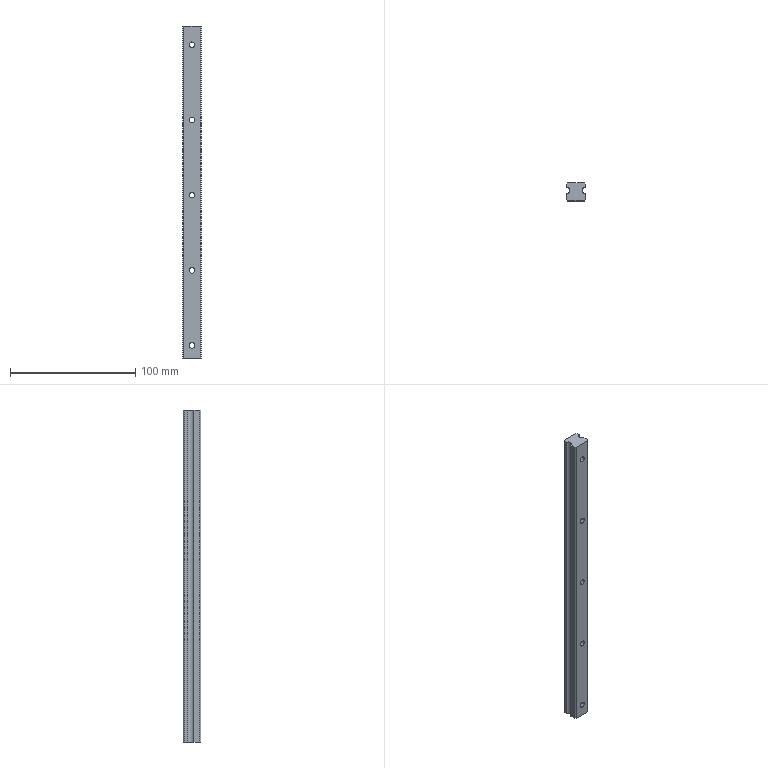Part | Creo | features CUT 6, CURVE 3, DATUM PLANE 3, COORDINATE SYSTEM 1, PATTERN 1, PROTRUSION 1 | 1 solid | 39 faces | box 15 x 14 x 265 mm | volume 47944 mm3 | cylinder 22 | plane 17 | commonest cylinder face diameters 4.5 x10 8 x10 5 x2
STEP:
#1=CARTESIAN_POINT('',(0.,0.,0.));
#2=DIRECTION('',(0.,0.,1.));
#3=DIRECTION('',(1.,0.,0.));
#4=AXIS2_PLACEMENT_3D('',#1,#2,#3);
#5=CARTESIAN_POINT('',(13.635,5.984,0.));
#6=VERTEX_POINT('',#5);
#7=CARTESIAN_POINT('',(13.635,10.984,0.));
#8=VERTEX_POINT('',#7);
#9=CARTESIAN_POINT('',(13.635,8.484,0.));
#10=DIRECTION('',(0.,0.,-1.));
#11=DIRECTION('',(0.00001575,-1.,0.));
#12=AXIS2_PLACEMENT_3D('',#9,#10,#11);
#13=CIRCLE('',#12,2.5);
#14=EDGE_CURVE('',#6,#8,#13,.T.);
#15=ORIENTED_EDGE('',*,*,#14,.T.);
#16=CARTESIAN_POINT('',(13.635,13.484,0.));
#17=VERTEX_POINT('',#16);
#18=CARTESIAN_POINT('',(13.635,10.984,0.));
#19=DIRECTION('',(-0.00001575,1.,0.));
#20=VECTOR('',#19,2.5);
#21=LINE('',#18,#20);
#22=EDGE_CURVE('',#8,#17,#21,.T.);
#23=ORIENTED_EDGE('',*,*,#22,.T.);
#24=CARTESIAN_POINT('',(12.635,14.484,0.));
#25=VERTEX_POINT('',#24);
#26=CARTESIAN_POINT('',(13.635,13.484,0.));
#27=DIRECTION('',(-0.7071,0.7071,0.));
#28=VECTOR('',#27,1.414);
#29=LINE('',#26,#28);
#30=EDGE_CURVE('',#17,#25,#29,.T.);
#31=ORIENTED_EDGE('',*,*,#30,.T.);
#32=CARTESIAN_POINT('',(-0.3654,14.484,0.));
#33=VERTEX_POINT('',#32);
#34=CARTESIAN_POINT('',(12.635,14.484,0.));
#35=DIRECTION('',(-1.,0.,0.));
#36=VECTOR('',#35,13.);
#37=LINE('',#34,#36);
#38=EDGE_CURVE('',#25,#33,#37,.T.);
#39=ORIENTED_EDGE('',*,*,#38,.T.);
#40=CARTESIAN_POINT('',(-1.365,13.484,0.));
#41=VERTEX_POINT('',#40);
#42=CARTESIAN_POINT('',(-0.3654,14.484,0.));
#43=DIRECTION('',(-0.7071,-0.7071,0.));
#44=VECTOR('',#43,1.414);
#45=LINE('',#42,#44);
#46=EDGE_CURVE('',#33,#41,#45,.T.);
#47=ORIENTED_EDGE('',*,*,#46,.T.);
#48=CARTESIAN_POINT('',(-1.365,10.984,0.));
#49=VERTEX_POINT('',#48);
#50=CARTESIAN_POINT('',(-1.365,13.484,0.));
#51=DIRECTION('',(0.00001575,-1.,0.));
#52=VECTOR('',#51,2.5);
#53=LINE('',#50,#52);
#54=EDGE_CURVE('',#41,#49,#53,.T.);
#55=ORIENTED_EDGE('',*,*,#54,.T.);
#56=CARTESIAN_POINT('',(-1.365,5.984,0.));
#57=VERTEX_POINT('',#56);
#58=CARTESIAN_POINT('',(-1.365,8.484,0.));
#59=DIRECTION('',(0.,0.,-1.));
#60=DIRECTION('',(-0.00001575,1.,0.));
#61=AXIS2_PLACEMENT_3D('',#58,#59,#60);
#62=CIRCLE('',#61,2.5);
#63=EDGE_CURVE('',#49,#57,#62,.T.);
#64=ORIENTED_EDGE('',*,*,#63,.T.);
#65=CARTESIAN_POINT('',(-1.365,1.484,0.));
#66=VERTEX_POINT('',#65);
#67=CARTESIAN_POINT('',(-1.365,5.984,0.));
#68=DIRECTION('',(0.00001575,-1.,0.));
#69=VECTOR('',#68,4.5);
#70=LINE('',#67,#69);
#71=EDGE_CURVE('',#57,#66,#70,.T.);
#72=ORIENTED_EDGE('',*,*,#71,.T.);
#73=CARTESIAN_POINT('',(-0.3654,0.4841,0.));
#74=VERTEX_POINT('',#73);
#75=CARTESIAN_POINT('',(-1.365,1.484,0.));
#76=DIRECTION('',(0.7071,-0.7071,0.));
#77=VECTOR('',#76,1.414);
#78=LINE('',#75,#77);
#79=EDGE_CURVE('',#66,#74,#78,.T.);
#80=ORIENTED_EDGE('',*,*,#79,.T.);
#81=CARTESIAN_POINT('',(12.635,0.4841,0.));
#82=VERTEX_POINT('',#81);
#83=CARTESIAN_POINT('',(-0.3654,0.4841,0.));
#84=DIRECTION('',(1.,0.,0.));
#85=VECTOR('',#84,13.);
#86=LINE('',#83,#85);
#87=EDGE_CURVE('',#74,#82,#86,.T.);
#88=ORIENTED_EDGE('',*,*,#87,.T.);
#89=CARTESIAN_POINT('',(13.635,1.484,0.));
#90=VERTEX_POINT('',#89);
#91=CARTESIAN_POINT('',(12.635,0.4841,0.));
#92=DIRECTION('',(0.7071,0.7071,0.));
#93=VECTOR('',#92,1.414);
#94=LINE('',#91,#93);
#95=EDGE_CURVE('',#82,#90,#94,.T.);
#96=ORIENTED_EDGE('',*,*,#95,.T.);
#97=CARTESIAN_POINT('',(13.635,1.484,0.));
#98=DIRECTION('',(-0.00001575,1.,0.));
#99=VECTOR('',#98,4.5);
#100=LINE('',#97,#99);
#101=EDGE_CURVE('',#90,#6,#100,.T.);
#102=ORIENTED_EDGE('',*,*,#101,.T.);
#103=EDGE_LOOP('',(#15,#23,#31,#39,#47,#55,#64,#72,#80,#88,#96,#102));
#104=FACE_OUTER_BOUND('',#103,.F.);
#105=CARTESIAN_POINT('',(0.,0.,0.));
#106=DIRECTION('',(0.,0.,1.));
#107=DIRECTION('',(1.,0.,0.));
#108=AXIS2_PLACEMENT_3D('',#105,#106,#107);
#109=PLANE('',#108);
#110=ADVANCED_FACE('',(#104),#109,.F.);
#111=ORIENTED_EDGE('',*,*,#14,.F.);
#112=CARTESIAN_POINT('',(13.635,5.984,265.));
#113=VERTEX_POINT('',#112);
#114=CARTESIAN_POINT('',(13.635,5.984,0.));
#115=DIRECTION('',(0.,0.,1.));
#116=VECTOR('',#115,265.);
#117=LINE('',#114,#116);
#118=EDGE_CURVE('',#6,#113,#117,.T.);
#119=ORIENTED_EDGE('',*,*,#118,.T.);
#120=CARTESIAN_POINT('',(13.635,10.984,265.));
#121=VERTEX_POINT('',#120);
#122=CARTESIAN_POINT('',(13.635,8.484,265.));
#123=DIRECTION('',(0.,0.,-1.));
#124=DIRECTION('',(0.00001575,-1.,0.));
#125=AXIS2_PLACEMENT_3D('',#122,#123,#124);
#126=CIRCLE('',#125,2.5);
#127=EDGE_CURVE('',#113,#121,#126,.T.);
#128=ORIENTED_EDGE('',*,*,#127,.T.);
#129=CARTESIAN_POINT('',(13.635,10.984,0.));
#130=DIRECTION('',(0.,0.,1.));
#131=VECTOR('',#130,265.);
#132=LINE('',#129,#131);
#133=EDGE_CURVE('',#8,#121,#132,.T.);
#134=ORIENTED_EDGE('',*,*,#133,.F.);
#135=EDGE_LOOP('',(#111,#119,#128,#134));
#136=FACE_OUTER_BOUND('',#135,.F.);
#137=CARTESIAN_POINT('',(13.635,8.484,0.));
#138=DIRECTION('',(0.,0.,1.));
#139=DIRECTION('',(1.,0.,0.));
#140=AXIS2_PLACEMENT_3D('',#137,#138,#139);
#141=CYLINDRICAL_SURFACE('',#140,2.5);
#142=ADVANCED_FACE('',(#136),#141,.F.);
#143=ORIENTED_EDGE('',*,*,#101,.F.);
#144=CARTESIAN_POINT('',(13.635,1.484,265.));
#145=VERTEX_POINT('',#144);
#146=CARTESIAN_POINT('',(13.635,1.484,0.));
#147=DIRECTION('',(0.,0.,1.));
#148=VECTOR('',#147,265.);
#149=LINE('',#146,#148);
#150=EDGE_CURVE('',#90,#145,#149,.T.);
#151=ORIENTED_EDGE('',*,*,#150,.T.);
#152=CARTESIAN_POINT('',(13.635,1.484,265.));
#153=DIRECTION('',(-0.00001575,1.,0.));
#154=VECTOR('',#153,4.5);
#155=LINE('',#152,#154);
#156=EDGE_CURVE('',#145,#113,#155,.T.);
#157=ORIENTED_EDGE('',*,*,#156,.T.);
#158=ORIENTED_EDGE('',*,*,#118,.F.);
#159=EDGE_LOOP('',(#143,#151,#157,#158));
#160=FACE_OUTER_BOUND('',#159,.F.);
#161=CARTESIAN_POINT('',(13.635,1.484,0.));
#162=DIRECTION('',(1.,0.00001575,0.));
#163=DIRECTION('',(-0.00001575,1.,0.));
#164=AXIS2_PLACEMENT_3D('',#161,#162,#163);
#165=PLANE('',#164);
#166=ADVANCED_FACE('',(#160),#165,.T.);
#167=ORIENTED_EDGE('',*,*,#95,.F.);
#168=CARTESIAN_POINT('',(12.635,0.4841,265.));
#169=VERTEX_POINT('',#168);
#170=CARTESIAN_POINT('',(12.635,0.4841,0.));
#171=DIRECTION('',(0.,0.,1.));
#172=VECTOR('',#171,265.);
#173=LINE('',#170,#172);
#174=EDGE_CURVE('',#82,#169,#173,.T.);
#175=ORIENTED_EDGE('',*,*,#174,.T.);
#176=CARTESIAN_POINT('',(12.635,0.4841,265.));
#177=DIRECTION('',(0.7071,0.7071,0.));
#178=VECTOR('',#177,1.414);
#179=LINE('',#176,#178);
#180=EDGE_CURVE('',#169,#145,#179,.T.);
#181=ORIENTED_EDGE('',*,*,#180,.T.);
#182=ORIENTED_EDGE('',*,*,#150,.F.);
#183=EDGE_LOOP('',(#167,#175,#181,#182));
#184=FACE_OUTER_BOUND('',#183,.F.);
#185=CARTESIAN_POINT('',(12.635,0.4841,0.));
#186=DIRECTION('',(0.7071,-0.7071,0.));
#187=DIRECTION('',(0.7071,0.7071,0.));
#188=AXIS2_PLACEMENT_3D('',#185,#186,#187);
#189=PLANE('',#188);
#190=ADVANCED_FACE('',(#184),#189,.T.);
#191=ORIENTED_EDGE('',*,*,#87,.F.);
#192=CARTESIAN_POINT('',(-0.3654,0.4841,265.));
#193=VERTEX_POINT('',#192);
#194=CARTESIAN_POINT('',(-0.3654,0.4841,0.));
#195=DIRECTION('',(0.,0.,1.));
#196=VECTOR('',#195,265.);
#197=LINE('',#194,#196);
#198=EDGE_CURVE('',#74,#193,#197,.T.);
#199=ORIENTED_EDGE('',*,*,#198,.T.);
#200=CARTESIAN_POINT('',(-0.3654,0.4841,265.));
#201=DIRECTION('',(1.,0.,0.));
#202=VECTOR('',#201,13.);
#203=LINE('',#200,#202);
#204=EDGE_CURVE('',#193,#169,#203,.T.);
#205=ORIENTED_EDGE('',*,*,#204,.T.);
#206=ORIENTED_EDGE('',*,*,#174,.F.);
#207=EDGE_LOOP('',(#191,#199,#205,#206));
#208=FACE_OUTER_BOUND('',#207,.F.);
#209=CARTESIAN_POINT('',(6.135,0.4841,7.75));
#210=VERTEX_POINT('',#209);
#211=CARTESIAN_POINT('',(6.135,0.4841,12.25));
#212=VERTEX_POINT('',#211);
#213=CARTESIAN_POINT('',(6.135,0.4841,10.));
#214=DIRECTION('',(0.,1.,0.));
#215=DIRECTION('',(0.,0.,-1.));
#216=AXIS2_PLACEMENT_3D('',#213,#214,#215);
#217=CIRCLE('',#216,2.25);
#218=EDGE_CURVE('',#210,#212,#217,.T.);
#219=ORIENTED_EDGE('',*,*,#218,.F.);
#220=CARTESIAN_POINT('',(6.135,0.4841,10.));
#221=DIRECTION('',(0.,1.,0.));
#222=DIRECTION('',(0.,0.,1.));
#223=AXIS2_PLACEMENT_3D('',#220,#221,#222);
#224=CIRCLE('',#223,2.25);
#225=EDGE_CURVE('',#212,#210,#224,.T.);
#226=ORIENTED_EDGE('',*,*,#225,.F.);
#227=EDGE_LOOP('',(#219,#226));
#228=FACE_BOUND('',#227,.F.);
#229=CARTESIAN_POINT('',(6.135,0.4841,67.75));
#230=VERTEX_POINT('',#229);
#231=CARTESIAN_POINT('',(6.135,0.4841,72.25));
#232=VERTEX_POINT('',#231);
#233=CARTESIAN_POINT('',(6.135,0.4841,70.));
#234=DIRECTION('',(0.,1.,0.));
#235=DIRECTION('',(0.,0.,-1.));
#236=AXIS2_PLACEMENT_3D('',#233,#234,#235);
#237=CIRCLE('',#236,2.25);
#238=EDGE_CURVE('',#230,#232,#237,.T.);
#239=ORIENTED_EDGE('',*,*,#238,.F.);
#240=CARTESIAN_POINT('',(6.135,0.4841,70.));
#241=DIRECTION('',(0.,1.,0.));
#242=DIRECTION('',(0.,0.,1.));
#243=AXIS2_PLACEMENT_3D('',#240,#241,#242);
#244=CIRCLE('',#243,2.25);
#245=EDGE_CURVE('',#232,#230,#244,.T.);
#246=ORIENTED_EDGE('',*,*,#245,.F.);
#247=EDGE_LOOP('',(#239,#246));
#248=FACE_BOUND('',#247,.F.);
#249=CARTESIAN_POINT('',(6.135,0.4841,127.75));
#250=VERTEX_POINT('',#249);
#251=CARTESIAN_POINT('',(6.135,0.4841,132.25));
#252=VERTEX_POINT('',#251);
#253=CARTESIAN_POINT('',(6.135,0.4841,130.));
#254=DIRECTION('',(0.,1.,0.));
#255=DIRECTION('',(0.,0.,-1.));
#256=AXIS2_PLACEMENT_3D('',#253,#254,#255);
#257=CIRCLE('',#256,2.25);
#258=EDGE_CURVE('',#250,#252,#257,.T.);
#259=ORIENTED_EDGE('',*,*,#258,.F.);
#260=CARTESIAN_POINT('',(6.135,0.4841,130.));
#261=DIRECTION('',(0.,1.,0.));
#262=DIRECTION('',(0.,0.,1.));
#263=AXIS2_PLACEMENT_3D('',#260,#261,#262);
#264=CIRCLE('',#263,2.25);
#265=EDGE_CURVE('',#252,#250,#264,.T.);
#266=ORIENTED_EDGE('',*,*,#265,.F.);
#267=EDGE_LOOP('',(#259,#266));
#268=FACE_BOUND('',#267,.F.);
#269=CARTESIAN_POINT('',(6.135,0.4841,187.75));
#270=VERTEX_POINT('',#269);
#271=CARTESIAN_POINT('',(6.135,0.4841,192.25));
#272=VERTEX_POINT('',#271);
#273=CARTESIAN_POINT('',(6.135,0.4841,190.));
#274=DIRECTION('',(0.,1.,0.));
#275=DIRECTION('',(0.,0.,-1.));
#276=AXIS2_PLACEMENT_3D('',#273,#274,#275);
#277=CIRCLE('',#276,2.25);
#278=EDGE_CURVE('',#270,#272,#277,.T.);
#279=ORIENTED_EDGE('',*,*,#278,.F.);
#280=CARTESIAN_POINT('',(6.135,0.4841,190.));
#281=DIRECTION('',(0.,1.,0.));
#282=DIRECTION('',(0.,0.,1.));
#283=AXIS2_PLACEMENT_3D('',#280,#281,#282);
#284=CIRCLE('',#283,2.25);
#285=EDGE_CURVE('',#272,#270,#284,.T.);
#286=ORIENTED_EDGE('',*,*,#285,.F.);
#287=EDGE_LOOP('',(#279,#286));
#288=FACE_BOUND('',#287,.F.);
#289=CARTESIAN_POINT('',(6.135,0.4841,247.75));
#290=VERTEX_POINT('',#289);
#291=CARTESIAN_POINT('',(6.135,0.4841,252.25));
#292=VERTEX_POINT('',#291);
#293=CARTESIAN_POINT('',(6.135,0.4841,250.));
#294=DIRECTION('',(0.,1.,0.));
#295=DIRECTION('',(0.,0.,-1.));
#296=AXIS2_PLACEMENT_3D('',#293,#294,#295);
#297=CIRCLE('',#296,2.25);
#298=EDGE_CURVE('',#290,#292,#297,.T.);
#299=ORIENTED_EDGE('',*,*,#298,.F.);
#300=CARTESIAN_POINT('',(6.135,0.4841,250.));
#301=DIRECTION('',(0.,1.,0.));
#302=DIRECTION('',(0.,0.,1.));
#303=AXIS2_PLACEMENT_3D('',#300,#301,#302);
#304=CIRCLE('',#303,2.25);
#305=EDGE_CURVE('',#292,#290,#304,.T.);
#306=ORIENTED_EDGE('',*,*,#305,.F.);
#307=EDGE_LOOP('',(#299,#306));
#308=FACE_BOUND('',#307,.F.);
#309=CARTESIAN_POINT('',(-0.3654,0.4841,0.));
#310=DIRECTION('',(0.,-1.,0.));
#311=DIRECTION('',(1.,0.,0.));
#312=AXIS2_PLACEMENT_3D('',#309,#310,#311);
#313=PLANE('',#312);
#314=ADVANCED_FACE('',(#208,#228,#248,#268,#288,#308),#313,.T.);
#315=ORIENTED_EDGE('',*,*,#79,.F.);
#316=CARTESIAN_POINT('',(-1.365,1.484,265.));
#317=VERTEX_POINT('',#316);
#318=CARTESIAN_POINT('',(-1.365,1.484,0.));
#319=DIRECTION('',(0.,0.,1.));
#320=VECTOR('',#319,265.);
#321=LINE('',#318,#320);
#322=EDGE_CURVE('',#66,#317,#321,.T.);
#323=ORIENTED_EDGE('',*,*,#322,.T.);
#324=CARTESIAN_POINT('',(-1.365,1.484,265.));
#325=DIRECTION('',(0.7071,-0.7071,0.));
#326=VECTOR('',#325,1.414);
#327=LINE('',#324,#326);
#328=EDGE_CURVE('',#317,#193,#327,.T.);
#329=ORIENTED_EDGE('',*,*,#328,.T.);
#330=ORIENTED_EDGE('',*,*,#198,.F.);
#331=EDGE_LOOP('',(#315,#323,#329,#330));
#332=FACE_OUTER_BOUND('',#331,.F.);
#333=CARTESIAN_POINT('',(-1.365,1.484,0.));
#334=DIRECTION('',(-0.7071,-0.7071,0.));
#335=DIRECTION('',(0.7071,-0.7071,0.));
#336=AXIS2_PLACEMENT_3D('',#333,#334,#335);
#337=PLANE('',#336);
#338=ADVANCED_FACE('',(#332),#337,.T.);
#339=ORIENTED_EDGE('',*,*,#71,.F.);
#340=CARTESIAN_POINT('',(-1.365,5.984,265.));
#341=VERTEX_POINT('',#340);
#342=CARTESIAN_POINT('',(-1.365,5.984,0.));
#343=DIRECTION('',(0.,0.,1.));
#344=VECTOR('',#343,265.);
#345=LINE('',#342,#344);
#346=EDGE_CURVE('',#57,#341,#345,.T.);
#347=ORIENTED_EDGE('',*,*,#346,.T.);
#348=CARTESIAN_POINT('',(-1.365,5.984,265.));
#349=DIRECTION('',(0.00001575,-1.,0.));
#350=VECTOR('',#349,4.5);
#351=LINE('',#348,#350);
#352=EDGE_CURVE('',#341,#317,#351,.T.);
#353=ORIENTED_EDGE('',*,*,#352,.T.);
#354=ORIENTED_EDGE('',*,*,#322,.F.);
#355=EDGE_LOOP('',(#339,#347,#353,#354));
#356=FACE_OUTER_BOUND('',#355,.F.);
#357=CARTESIAN_POINT('',(-1.365,5.984,0.));
#358=DIRECTION('',(-1.,-0.00001575,0.));
#359=DIRECTION('',(0.00001575,-1.,0.));
#360=AXIS2_PLACEMENT_3D('',#357,#358,#359);
#361=PLANE('',#360);
#362=ADVANCED_FACE('',(#356),#361,.T.);
#363=ORIENTED_EDGE('',*,*,#63,.F.);
#364=CARTESIAN_POINT('',(-1.365,10.984,265.));
#365=VERTEX_POINT('',#364);
#366=CARTESIAN_POINT('',(-1.365,10.984,0.));
#367=DIRECTION('',(0.,0.,1.));
#368=VECTOR('',#367,265.);
#369=LINE('',#366,#368);
#370=EDGE_CURVE('',#49,#365,#369,.T.);
#371=ORIENTED_EDGE('',*,*,#370,.T.);
#372=CARTESIAN_POINT('',(-1.365,8.484,265.));
#373=DIRECTION('',(0.,0.,-1.));
#374=DIRECTION('',(-0.00001575,1.,0.));
#375=AXIS2_PLACEMENT_3D('',#372,#373,#374);
#376=CIRCLE('',#375,2.5);
#377=EDGE_CURVE('',#365,#341,#376,.T.);
#378=ORIENTED_EDGE('',*,*,#377,.T.);
#379=ORIENTED_EDGE('',*,*,#346,.F.);
#380=EDGE_LOOP('',(#363,#371,#378,#379));
#381=FACE_OUTER_BOUND('',#380,.F.);
#382=CARTESIAN_POINT('',(-1.365,8.484,0.));
#383=DIRECTION('',(0.,0.,1.));
#384=DIRECTION('',(1.,0.,0.));
#385=AXIS2_PLACEMENT_3D('',#382,#383,#384);
#386=CYLINDRICAL_SURFACE('',#385,2.5);
#387=ADVANCED_FACE('',(#381),#386,.F.);
#388=ORIENTED_EDGE('',*,*,#54,.F.);
#389=CARTESIAN_POINT('',(-1.365,13.484,265.));
#390=VERTEX_POINT('',#389);
#391=CARTESIAN_POINT('',(-1.365,13.484,0.));
#392=DIRECTION('',(0.,0.,1.));
#393=VECTOR('',#392,265.);
#394=LINE('',#391,#393);
#395=EDGE_CURVE('',#41,#390,#394,.T.);
#396=ORIENTED_EDGE('',*,*,#395,.T.);
#397=CARTESIAN_POINT('',(-1.365,13.484,265.));
#398=DIRECTION('',(0.00001575,-1.,0.));
#399=VECTOR('',#398,2.5);
#400=LINE('',#397,#399);
#401=EDGE_CURVE('',#390,#365,#400,.T.);
#402=ORIENTED_EDGE('',*,*,#401,.T.);
#403=ORIENTED_EDGE('',*,*,#370,.F.);
#404=EDGE_LOOP('',(#388,#396,#402,#403));
#405=FACE_OUTER_BOUND('',#404,.F.);
#406=CARTESIAN_POINT('',(-1.365,13.484,0.));
#407=DIRECTION('',(-1.,-0.00001575,0.));
#408=DIRECTION('',(0.00001575,-1.,0.));
#409=AXIS2_PLACEMENT_3D('',#406,#407,#408);
#410=PLANE('',#409);
#411=ADVANCED_FACE('',(#405),#410,.T.);
#412=ORIENTED_EDGE('',*,*,#46,.F.);
#413=CARTESIAN_POINT('',(-0.3654,14.484,265.));
#414=VERTEX_POINT('',#413);
#415=CARTESIAN_POINT('',(-0.3654,14.484,0.));
#416=DIRECTION('',(0.,0.,1.));
#417=VECTOR('',#416,265.);
#418=LINE('',#415,#417);
#419=EDGE_CURVE('',#33,#414,#418,.T.);
#420=ORIENTED_EDGE('',*,*,#419,.T.);
#421=CARTESIAN_POINT('',(-0.3654,14.484,265.));
#422=DIRECTION('',(-0.7071,-0.7071,0.));
#423=VECTOR('',#422,1.414);
#424=LINE('',#421,#423);
#425=EDGE_CURVE('',#414,#390,#424,.T.);
#426=ORIENTED_EDGE('',*,*,#425,.T.);
#427=ORIENTED_EDGE('',*,*,#395,.F.);
#428=EDGE_LOOP('',(#412,#420,#426,#427));
#429=FACE_OUTER_BOUND('',#428,.F.);
#430=CARTESIAN_POINT('',(-0.3654,14.484,0.));
#431=DIRECTION('',(-0.7071,0.7071,0.));
#432=DIRECTION('',(-0.7071,-0.7071,0.));
#433=AXIS2_PLACEMENT_3D('',#430,#431,#432);
#434=PLANE('',#433);
#435=ADVANCED_FACE('',(#429),#434,.T.);
#436=ORIENTED_EDGE('',*,*,#38,.F.);
#437=CARTESIAN_POINT('',(12.635,14.484,265.));
#438=VERTEX_POINT('',#437);
#439=CARTESIAN_POINT('',(12.635,14.484,0.));
#440=DIRECTION('',(0.,0.,1.));
#441=VECTOR('',#440,265.);
#442=LINE('',#439,#441);
#443=EDGE_CURVE('',#25,#438,#442,.T.);
#444=ORIENTED_EDGE('',*,*,#443,.T.);
#445=CARTESIAN_POINT('',(12.635,14.484,265.));
#446=DIRECTION('',(-1.,0.,0.));
#447=VECTOR('',#446,13.);
#448=LINE('',#445,#447);
#449=EDGE_CURVE('',#438,#414,#448,.T.);
#450=ORIENTED_EDGE('',*,*,#449,.T.);
#451=ORIENTED_EDGE('',*,*,#419,.F.);
#452=EDGE_LOOP('',(#436,#444,#450,#451));
#453=FACE_OUTER_BOUND('',#452,.F.);
#454=CARTESIAN_POINT('',(6.135,14.484,6.));
#455=VERTEX_POINT('',#454);
#456=CARTESIAN_POINT('',(6.135,14.484,14.));
#457=VERTEX_POINT('',#456);
#458=CARTESIAN_POINT('',(6.135,14.484,10.));
#459=DIRECTION('',(0.,1.,0.));
#460=DIRECTION('',(0.,0.,-1.));
#461=AXIS2_PLACEMENT_3D('',#458,#459,#460);
#462=CIRCLE('',#461,4.);
#463=EDGE_CURVE('',#455,#457,#462,.T.);
#464=ORIENTED_EDGE('',*,*,#463,.T.);
#465=CARTESIAN_POINT('',(6.135,14.484,10.));
#466=DIRECTION('',(0.,1.,0.));
#467=DIRECTION('',(0.,0.,1.));
#468=AXIS2_PLACEMENT_3D('',#465,#466,#467);
#469=CIRCLE('',#468,4.);
#470=EDGE_CURVE('',#457,#455,#469,.T.);
#471=ORIENTED_EDGE('',*,*,#470,.T.);
#472=EDGE_LOOP('',(#464,#471));
#473=FACE_BOUND('',#472,.F.);
#474=CARTESIAN_POINT('',(6.135,14.484,66.));
#475=VERTEX_POINT('',#474);
#476=CARTESIAN_POINT('',(6.135,14.484,74.));
#477=VERTEX_POINT('',#476);
#478=CARTESIAN_POINT('',(6.135,14.484,70.));
#479=DIRECTION('',(0.,1.,0.));
#480=DIRECTION('',(0.,0.,-1.));
#481=AXIS2_PLACEMENT_3D('',#478,#479,#480);
#482=CIRCLE('',#481,4.);
#483=EDGE_CURVE('',#475,#477,#482,.T.);
#484=ORIENTED_EDGE('',*,*,#483,.T.);
#485=CARTESIAN_POINT('',(6.135,14.484,70.));
#486=DIRECTION('',(0.,1.,0.));
#487=DIRECTION('',(0.,0.,1.));
#488=AXIS2_PLACEMENT_3D('',#485,#486,#487);
#489=CIRCLE('',#488,4.);
#490=EDGE_CURVE('',#477,#475,#489,.T.);
#491=ORIENTED_EDGE('',*,*,#490,.T.);
#492=EDGE_LOOP('',(#484,#491));
#493=FACE_BOUND('',#492,.F.);
#494=CARTESIAN_POINT('',(6.135,14.484,126.));
#495=VERTEX_POINT('',#494);
#496=CARTESIAN_POINT('',(6.135,14.484,134.));
#497=VERTEX_POINT('',#496);
#498=CARTESIAN_POINT('',(6.135,14.484,130.));
#499=DIRECTION('',(0.,1.,0.));
#500=DIRECTION('',(0.,0.,-1.));
#501=AXIS2_PLACEMENT_3D('',#498,#499,#500);
#502=CIRCLE('',#501,4.);
#503=EDGE_CURVE('',#495,#497,#502,.T.);
#504=ORIENTED_EDGE('',*,*,#503,.T.);
#505=CARTESIAN_POINT('',(6.135,14.484,130.));
#506=DIRECTION('',(0.,1.,0.));
#507=DIRECTION('',(0.,0.,1.));
#508=AXIS2_PLACEMENT_3D('',#505,#506,#507);
#509=CIRCLE('',#508,4.);
#510=EDGE_CURVE('',#497,#495,#509,.T.);
#511=ORIENTED_EDGE('',*,*,#510,.T.);
#512=EDGE_LOOP('',(#504,#511));
#513=FACE_BOUND('',#512,.F.);
#514=CARTESIAN_POINT('',(6.135,14.484,186.));
#515=VERTEX_POINT('',#514);
#516=CARTESIAN_POINT('',(6.135,14.484,194.));
#517=VERTEX_POINT('',#516);
#518=CARTESIAN_POINT('',(6.135,14.484,190.));
#519=DIRECTION('',(0.,1.,0.));
#520=DIRECTION('',(0.,0.,-1.));
#521=AXIS2_PLACEMENT_3D('',#518,#519,#520);
#522=CIRCLE('',#521,4.);
#523=EDGE_CURVE('',#515,#517,#522,.T.);
#524=ORIENTED_EDGE('',*,*,#523,.T.);
#525=CARTESIAN_POINT('',(6.135,14.484,190.));
#526=DIRECTION('',(0.,1.,0.));
#527=DIRECTION('',(0.,0.,1.));
#528=AXIS2_PLACEMENT_3D('',#525,#526,#527);
#529=CIRCLE('',#528,4.);
#530=EDGE_CURVE('',#517,#515,#529,.T.);
#531=ORIENTED_EDGE('',*,*,#530,.T.);
#532=EDGE_LOOP('',(#524,#531));
#533=FACE_BOUND('',#532,.F.);
#534=CARTESIAN_POINT('',(6.135,14.484,246.));
#535=VERTEX_POINT('',#534);
#536=CARTESIAN_POINT('',(6.135,14.484,254.));
#537=VERTEX_POINT('',#536);
#538=CARTESIAN_POINT('',(6.135,14.484,250.));
#539=DIRECTION('',(0.,1.,0.));
#540=DIRECTION('',(0.,0.,-1.));
#541=AXIS2_PLACEMENT_3D('',#538,#539,#540);
#542=CIRCLE('',#541,4.);
#543=EDGE_CURVE('',#535,#537,#542,.T.);
#544=ORIENTED_EDGE('',*,*,#543,.T.);
#545=CARTESIAN_POINT('',(6.135,14.484,250.));
#546=DIRECTION('',(0.,1.,0.));
#547=DIRECTION('',(0.,0.,1.));
#548=AXIS2_PLACEMENT_3D('',#545,#546,#547);
#549=CIRCLE('',#548,4.);
#550=EDGE_CURVE('',#537,#535,#549,.T.);
#551=ORIENTED_EDGE('',*,*,#550,.T.);
#552=EDGE_LOOP('',(#544,#551));
#553=FACE_BOUND('',#552,.F.);
#554=CARTESIAN_POINT('',(12.635,14.484,0.));
#555=DIRECTION('',(0.,1.,0.));
#556=DIRECTION('',(-1.,0.,0.));
#557=AXIS2_PLACEMENT_3D('',#554,#555,#556);
#558=PLANE('',#557);
#559=ADVANCED_FACE('',(#453,#473,#493,#513,#533,#553),#558,.T.);
#560=ORIENTED_EDGE('',*,*,#30,.F.);
#561=CARTESIAN_POINT('',(13.635,13.484,265.));
#562=VERTEX_POINT('',#561);
#563=CARTESIAN_POINT('',(13.635,13.484,0.));
#564=DIRECTION('',(0.,0.,1.));
#565=VECTOR('',#564,265.);
#566=LINE('',#563,#565);
#567=EDGE_CURVE('',#17,#562,#566,.T.);
#568=ORIENTED_EDGE('',*,*,#567,.T.);
#569=CARTESIAN_POINT('',(13.635,13.484,265.));
#570=DIRECTION('',(-0.7071,0.7071,0.));
#571=VECTOR('',#570,1.414);
#572=LINE('',#569,#571);
#573=EDGE_CURVE('',#562,#438,#572,.T.);
#574=ORIENTED_EDGE('',*,*,#573,.T.);
#575=ORIENTED_EDGE('',*,*,#443,.F.);
#576=EDGE_LOOP('',(#560,#568,#574,#575));
#577=FACE_OUTER_BOUND('',#576,.F.);
#578=CARTESIAN_POINT('',(13.635,13.484,0.));
#579=DIRECTION('',(0.7071,0.7071,0.));
#580=DIRECTION('',(-0.7071,0.7071,0.));
#581=AXIS2_PLACEMENT_3D('',#578,#579,#580);
#582=PLANE('',#581);
#583=ADVANCED_FACE('',(#577),#582,.T.);
#584=ORIENTED_EDGE('',*,*,#22,.F.);
#585=ORIENTED_EDGE('',*,*,#133,.T.);
#586=CARTESIAN_POINT('',(13.635,10.984,265.));
#587=DIRECTION('',(-0.00001575,1.,0.));
#588=VECTOR('',#587,2.5);
#589=LINE('',#586,#588);
#590=EDGE_CURVE('',#121,#562,#589,.T.);
#591=ORIENTED_EDGE('',*,*,#590,.T.);
#592=ORIENTED_EDGE('',*,*,#567,.F.);
#593=EDGE_LOOP('',(#584,#585,#591,#592));
#594=FACE_OUTER_BOUND('',#593,.F.);
#595=CARTESIAN_POINT('',(13.635,10.984,0.));
#596=DIRECTION('',(1.,0.00001575,0.));
#597=DIRECTION('',(-0.00001575,1.,0.));
#598=AXIS2_PLACEMENT_3D('',#595,#596,#597);
#599=PLANE('',#598);
#600=ADVANCED_FACE('',(#594),#599,.T.);
#601=ORIENTED_EDGE('',*,*,#127,.F.);
#602=ORIENTED_EDGE('',*,*,#156,.F.);
#603=ORIENTED_EDGE('',*,*,#180,.F.);
#604=ORIENTED_EDGE('',*,*,#204,.F.);
#605=ORIENTED_EDGE('',*,*,#328,.F.);
#606=ORIENTED_EDGE('',*,*,#352,.F.);
#607=ORIENTED_EDGE('',*,*,#377,.F.);
#608=ORIENTED_EDGE('',*,*,#401,.F.);
#609=ORIENTED_EDGE('',*,*,#425,.F.);
#610=ORIENTED_EDGE('',*,*,#449,.F.);
#611=ORIENTED_EDGE('',*,*,#573,.F.);
#612=ORIENTED_EDGE('',*,*,#590,.F.);
#613=EDGE_LOOP('',(#601,#602,#603,#604,#605,#606,#607,#608,#609,#610,#611,#612));
#614=FACE_OUTER_BOUND('',#613,.F.);
#615=CARTESIAN_POINT('',(0.,0.,265.));
#616=DIRECTION('',(0.,0.,1.));
#617=DIRECTION('',(1.,0.,0.));
#618=AXIS2_PLACEMENT_3D('',#615,#616,#617);
#619=PLANE('',#618);
#620=ADVANCED_FACE('',(#614),#619,.T.);
#621=ORIENTED_EDGE('',*,*,#463,.F.);
#622=CARTESIAN_POINT('',(6.135,9.484,6.));
#623=VERTEX_POINT('',#622);
#624=CARTESIAN_POINT('',(6.135,14.484,6.));
#625=DIRECTION('',(0.,-1.,0.));
#626=VECTOR('',#625,5.);
#627=LINE('',#624,#626);
#628=EDGE_CURVE('',#455,#623,#627,.T.);
#629=ORIENTED_EDGE('',*,*,#628,.T.);
#630=CARTESIAN_POINT('',(6.135,9.484,14.));
#631=VERTEX_POINT('',#630);
#632=CARTESIAN_POINT('',(6.135,9.484,10.));
#633=DIRECTION('',(0.,1.,0.));
#634=DIRECTION('',(0.,0.,-1.));
#635=AXIS2_PLACEMENT_3D('',#632,#633,#634);
#636=CIRCLE('',#635,4.);
#637=EDGE_CURVE('',#623,#631,#636,.T.);
#638=ORIENTED_EDGE('',*,*,#637,.T.);
#639=CARTESIAN_POINT('',(6.135,14.484,14.));
#640=DIRECTION('',(0.,-1.,0.));
#641=VECTOR('',#640,5.);
#642=LINE('',#639,#641);
#643=EDGE_CURVE('',#457,#631,#642,.T.);
#644=ORIENTED_EDGE('',*,*,#643,.F.);
#645=EDGE_LOOP('',(#621,#629,#638,#644));
#646=FACE_OUTER_BOUND('',#645,.F.);
#647=CARTESIAN_POINT('',(6.135,14.484,10.));
#648=DIRECTION('',(0.,1.,0.));
#649=DIRECTION('',(0.,0.,-1.));
#650=AXIS2_PLACEMENT_3D('',#647,#648,#649);
#651=CYLINDRICAL_SURFACE('',#650,4.);
#652=ADVANCED_FACE('',(#646),#651,.F.);
#653=ORIENTED_EDGE('',*,*,#470,.F.);
#654=ORIENTED_EDGE('',*,*,#643,.T.);
#655=CARTESIAN_POINT('',(6.135,9.484,10.));
#656=DIRECTION('',(0.,1.,0.));
#657=DIRECTION('',(0.,0.,1.));
#658=AXIS2_PLACEMENT_3D('',#655,#656,#657);
#659=CIRCLE('',#658,4.);
#660=EDGE_CURVE('',#631,#623,#659,.T.);
#661=ORIENTED_EDGE('',*,*,#660,.T.);
#662=ORIENTED_EDGE('',*,*,#628,.F.);
#663=EDGE_LOOP('',(#653,#654,#661,#662));
#664=FACE_OUTER_BOUND('',#663,.F.);
#665=CARTESIAN_POINT('',(6.135,14.484,10.));
#666=DIRECTION('',(0.,1.,0.));
#667=DIRECTION('',(0.,0.,-1.));
#668=AXIS2_PLACEMENT_3D('',#665,#666,#667);
#669=CYLINDRICAL_SURFACE('',#668,4.);
#670=ADVANCED_FACE('',(#664),#669,.F.);
#671=ORIENTED_EDGE('',*,*,#637,.F.);
#672=ORIENTED_EDGE('',*,*,#660,.F.);
#673=EDGE_LOOP('',(#671,#672));
#674=FACE_OUTER_BOUND('',#673,.F.);
#675=CARTESIAN_POINT('',(6.135,9.484,7.75));
#676=VERTEX_POINT('',#675);
#677=CARTESIAN_POINT('',(6.135,9.484,12.25));
#678=VERTEX_POINT('',#677);
#679=CARTESIAN_POINT('',(6.135,9.484,10.));
#680=DIRECTION('',(0.,1.,0.));
#681=DIRECTION('',(0.,0.,-1.));
#682=AXIS2_PLACEMENT_3D('',#679,#680,#681);
#683=CIRCLE('',#682,2.25);
#684=EDGE_CURVE('',#676,#678,#683,.T.);
#685=ORIENTED_EDGE('',*,*,#684,.T.);
#686=CARTESIAN_POINT('',(6.135,9.484,10.));
#687=DIRECTION('',(0.,1.,0.));
#688=DIRECTION('',(0.,0.,1.));
#689=AXIS2_PLACEMENT_3D('',#686,#687,#688);
#690=CIRCLE('',#689,2.25);
#691=EDGE_CURVE('',#678,#676,#690,.T.);
#692=ORIENTED_EDGE('',*,*,#691,.T.);
#693=EDGE_LOOP('',(#685,#692));
#694=FACE_BOUND('',#693,.F.);
#695=CARTESIAN_POINT('',(0.,9.484,0.));
#696=DIRECTION('',(0.,1.,0.));
#697=DIRECTION('',(0.,0.,-1.));
#698=AXIS2_PLACEMENT_3D('',#695,#696,#697);
#699=PLANE('',#698);
#700=ADVANCED_FACE('',(#674,#694),#699,.T.);
#701=CARTESIAN_POINT('',(6.135,9.484,66.));
#702=VERTEX_POINT('',#701);
#703=CARTESIAN_POINT('',(6.135,9.484,74.));
#704=VERTEX_POINT('',#703);
#705=CARTESIAN_POINT('',(6.135,9.484,70.));
#706=DIRECTION('',(0.,1.,0.));
#707=DIRECTION('',(0.,0.,-1.));
#708=AXIS2_PLACEMENT_3D('',#705,#706,#707);
#709=CIRCLE('',#708,4.);
#710=EDGE_CURVE('',#702,#704,#709,.T.);
#711=ORIENTED_EDGE('',*,*,#710,.F.);
#712=CARTESIAN_POINT('',(6.135,9.484,70.));
#713=DIRECTION('',(0.,1.,0.));
#714=DIRECTION('',(0.,0.,1.));
#715=AXIS2_PLACEMENT_3D('',#712,#713,#714);
#716=CIRCLE('',#715,4.);
#717=EDGE_CURVE('',#704,#702,#716,.T.);
#718=ORIENTED_EDGE('',*,*,#717,.F.);
#719=EDGE_LOOP('',(#711,#718));
#720=FACE_OUTER_BOUND('',#719,.F.);
#721=CARTESIAN_POINT('',(6.135,9.484,67.75));
#722=VERTEX_POINT('',#721);
#723=CARTESIAN_POINT('',(6.135,9.484,72.25));
#724=VERTEX_POINT('',#723);
#725=CARTESIAN_POINT('',(6.135,9.484,70.));
#726=DIRECTION('',(0.,1.,0.));
#727=DIRECTION('',(0.,0.,-1.));
#728=AXIS2_PLACEMENT_3D('',#725,#726,#727);
#729=CIRCLE('',#728,2.25);
#730=EDGE_CURVE('',#722,#724,#729,.T.);
#731=ORIENTED_EDGE('',*,*,#730,.T.);
#732=CARTESIAN_POINT('',(6.135,9.484,70.));
#733=DIRECTION('',(0.,1.,0.));
#734=DIRECTION('',(0.,0.,1.));
#735=AXIS2_PLACEMENT_3D('',#732,#733,#734);
#736=CIRCLE('',#735,2.25);
#737=EDGE_CURVE('',#724,#722,#736,.T.);
#738=ORIENTED_EDGE('',*,*,#737,.T.);
#739=EDGE_LOOP('',(#731,#738));
#740=FACE_BOUND('',#739,.F.);
#741=CARTESIAN_POINT('',(0.,9.484,0.));
#742=DIRECTION('',(0.,1.,0.));
#743=DIRECTION('',(0.,0.,-1.));
#744=AXIS2_PLACEMENT_3D('',#741,#742,#743);
#745=PLANE('',#744);
#746=ADVANCED_FACE('',(#720,#740),#745,.T.);
#747=CARTESIAN_POINT('',(6.135,9.484,126.));
#748=VERTEX_POINT('',#747);
#749=CARTESIAN_POINT('',(6.135,9.484,134.));
#750=VERTEX_POINT('',#749);
#751=CARTESIAN_POINT('',(6.135,9.484,130.));
#752=DIRECTION('',(0.,1.,0.));
#753=DIRECTION('',(0.,0.,-1.));
#754=AXIS2_PLACEMENT_3D('',#751,#752,#753);
#755=CIRCLE('',#754,4.);
#756=EDGE_CURVE('',#748,#750,#755,.T.);
#757=ORIENTED_EDGE('',*,*,#756,.F.);
#758=CARTESIAN_POINT('',(6.135,9.484,130.));
#759=DIRECTION('',(0.,1.,0.));
#760=DIRECTION('',(0.,0.,1.));
#761=AXIS2_PLACEMENT_3D('',#758,#759,#760);
#762=CIRCLE('',#761,4.);
#763=EDGE_CURVE('',#750,#748,#762,.T.);
#764=ORIENTED_EDGE('',*,*,#763,.F.);
#765=EDGE_LOOP('',(#757,#764));
#766=FACE_OUTER_BOUND('',#765,.F.);
#767=CARTESIAN_POINT('',(6.135,9.484,127.75));
#768=VERTEX_POINT('',#767);
#769=CARTESIAN_POINT('',(6.135,9.484,132.25));
#770=VERTEX_POINT('',#769);
#771=CARTESIAN_POINT('',(6.135,9.484,130.));
#772=DIRECTION('',(0.,1.,0.));
#773=DIRECTION('',(0.,0.,-1.));
#774=AXIS2_PLACEMENT_3D('',#771,#772,#773);
#775=CIRCLE('',#774,2.25);
#776=EDGE_CURVE('',#768,#770,#775,.T.);
#777=ORIENTED_EDGE('',*,*,#776,.T.);
#778=CARTESIAN_POINT('',(6.135,9.484,130.));
#779=DIRECTION('',(0.,1.,0.));
#780=DIRECTION('',(0.,0.,1.));
#781=AXIS2_PLACEMENT_3D('',#778,#779,#780);
#782=CIRCLE('',#781,2.25);
#783=EDGE_CURVE('',#770,#768,#782,.T.);
#784=ORIENTED_EDGE('',*,*,#783,.T.);
#785=EDGE_LOOP('',(#777,#784));
#786=FACE_BOUND('',#785,.F.);
#787=CARTESIAN_POINT('',(0.,9.484,0.));
#788=DIRECTION('',(0.,1.,0.));
#789=DIRECTION('',(0.,0.,-1.));
#790=AXIS2_PLACEMENT_3D('',#787,#788,#789);
#791=PLANE('',#790);
#792=ADVANCED_FACE('',(#766,#786),#791,.T.);
#793=CARTESIAN_POINT('',(6.135,9.484,186.));
#794=VERTEX_POINT('',#793);
#795=CARTESIAN_POINT('',(6.135,9.484,194.));
#796=VERTEX_POINT('',#795);
#797=CARTESIAN_POINT('',(6.135,9.484,190.));
#798=DIRECTION('',(0.,1.,0.));
#799=DIRECTION('',(0.,0.,-1.));
#800=AXIS2_PLACEMENT_3D('',#797,#798,#799);
#801=CIRCLE('',#800,4.);
#802=EDGE_CURVE('',#794,#796,#801,.T.);
#803=ORIENTED_EDGE('',*,*,#802,.F.);
#804=CARTESIAN_POINT('',(6.135,9.484,190.));
#805=DIRECTION('',(0.,1.,0.));
#806=DIRECTION('',(0.,0.,1.));
#807=AXIS2_PLACEMENT_3D('',#804,#805,#806);
#808=CIRCLE('',#807,4.);
#809=EDGE_CURVE('',#796,#794,#808,.T.);
#810=ORIENTED_EDGE('',*,*,#809,.F.);
#811=EDGE_LOOP('',(#803,#810));
#812=FACE_OUTER_BOUND('',#811,.F.);
#813=CARTESIAN_POINT('',(6.135,9.484,187.75));
#814=VERTEX_POINT('',#813);
#815=CARTESIAN_POINT('',(6.135,9.484,192.25));
#816=VERTEX_POINT('',#815);
#817=CARTESIAN_POINT('',(6.135,9.484,190.));
#818=DIRECTION('',(0.,1.,0.));
#819=DIRECTION('',(0.,0.,-1.));
#820=AXIS2_PLACEMENT_3D('',#817,#818,#819);
#821=CIRCLE('',#820,2.25);
#822=EDGE_CURVE('',#814,#816,#821,.T.);
#823=ORIENTED_EDGE('',*,*,#822,.T.);
#824=CARTESIAN_POINT('',(6.135,9.484,190.));
#825=DIRECTION('',(0.,1.,0.));
#826=DIRECTION('',(0.,0.,1.));
#827=AXIS2_PLACEMENT_3D('',#824,#825,#826);
#828=CIRCLE('',#827,2.25);
#829=EDGE_CURVE('',#816,#814,#828,.T.);
#830=ORIENTED_EDGE('',*,*,#829,.T.);
#831=EDGE_LOOP('',(#823,#830));
#832=FACE_BOUND('',#831,.F.);
#833=CARTESIAN_POINT('',(0.,9.484,0.));
#834=DIRECTION('',(0.,1.,0.));
#835=DIRECTION('',(0.,0.,-1.));
#836=AXIS2_PLACEMENT_3D('',#833,#834,#835);
#837=PLANE('',#836);
#838=ADVANCED_FACE('',(#812,#832),#837,.T.);
#839=CARTESIAN_POINT('',(6.135,9.484,246.));
#840=VERTEX_POINT('',#839);
#841=CARTESIAN_POINT('',(6.135,9.484,254.));
#842=VERTEX_POINT('',#841);
#843=CARTESIAN_POINT('',(6.135,9.484,250.));
#844=DIRECTION('',(0.,1.,0.));
#845=DIRECTION('',(0.,0.,-1.));
#846=AXIS2_PLACEMENT_3D('',#843,#844,#845);
#847=CIRCLE('',#846,4.);
#848=EDGE_CURVE('',#840,#842,#847,.T.);
#849=ORIENTED_EDGE('',*,*,#848,.F.);
#850=CARTESIAN_POINT('',(6.135,9.484,250.));
#851=DIRECTION('',(0.,1.,0.));
#852=DIRECTION('',(0.,0.,1.));
#853=AXIS2_PLACEMENT_3D('',#850,#851,#852);
#854=CIRCLE('',#853,4.);
#855=EDGE_CURVE('',#842,#840,#854,.T.);
#856=ORIENTED_EDGE('',*,*,#855,.F.);
#857=EDGE_LOOP('',(#849,#856));
#858=FACE_OUTER_BOUND('',#857,.F.);
#859=CARTESIAN_POINT('',(6.135,9.484,247.75));
#860=VERTEX_POINT('',#859);
#861=CARTESIAN_POINT('',(6.135,9.484,252.25));
#862=VERTEX_POINT('',#861);
#863=CARTESIAN_POINT('',(6.135,9.484,250.));
#864=DIRECTION('',(0.,1.,0.));
#865=DIRECTION('',(0.,0.,-1.));
#866=AXIS2_PLACEMENT_3D('',#863,#864,#865);
#867=CIRCLE('',#866,2.25);
#868=EDGE_CURVE('',#860,#862,#867,.T.);
#869=ORIENTED_EDGE('',*,*,#868,.T.);
#870=CARTESIAN_POINT('',(6.135,9.484,250.));
#871=DIRECTION('',(0.,1.,0.));
#872=DIRECTION('',(0.,0.,1.));
#873=AXIS2_PLACEMENT_3D('',#870,#871,#872);
#874=CIRCLE('',#873,2.25);
#875=EDGE_CURVE('',#862,#860,#874,.T.);
#876=ORIENTED_EDGE('',*,*,#875,.T.);
#877=EDGE_LOOP('',(#869,#876));
#878=FACE_BOUND('',#877,.F.);
#879=CARTESIAN_POINT('',(0.,9.484,0.));
#880=DIRECTION('',(0.,1.,0.));
#881=DIRECTION('',(0.,0.,-1.));
#882=AXIS2_PLACEMENT_3D('',#879,#880,#881);
#883=PLANE('',#882);
#884=ADVANCED_FACE('',(#858,#878),#883,.T.);
#885=ORIENTED_EDGE('',*,*,#483,.F.);
#886=CARTESIAN_POINT('',(6.135,14.484,66.));
#887=DIRECTION('',(0.,-1.,0.));
#888=VECTOR('',#887,5.);
#889=LINE('',#886,#888);
#890=EDGE_CURVE('',#475,#702,#889,.T.);
#891=ORIENTED_EDGE('',*,*,#890,.T.);
#892=ORIENTED_EDGE('',*,*,#710,.T.);
#893=CARTESIAN_POINT('',(6.135,14.484,74.));
#894=DIRECTION('',(0.,-1.,0.));
#895=VECTOR('',#894,5.);
#896=LINE('',#893,#895);
#897=EDGE_CURVE('',#477,#704,#896,.T.);
#898=ORIENTED_EDGE('',*,*,#897,.F.);
#899=EDGE_LOOP('',(#885,#891,#892,#898));
#900=FACE_OUTER_BOUND('',#899,.F.);
#901=CARTESIAN_POINT('',(6.135,14.484,70.));
#902=DIRECTION('',(0.,1.,0.));
#903=DIRECTION('',(0.,0.,-1.));
#904=AXIS2_PLACEMENT_3D('',#901,#902,#903);
#905=CYLINDRICAL_SURFACE('',#904,4.);
#906=ADVANCED_FACE('',(#900),#905,.F.);
#907=ORIENTED_EDGE('',*,*,#490,.F.);
#908=ORIENTED_EDGE('',*,*,#897,.T.);
#909=ORIENTED_EDGE('',*,*,#717,.T.);
#910=ORIENTED_EDGE('',*,*,#890,.F.);
#911=EDGE_LOOP('',(#907,#908,#909,#910));
#912=FACE_OUTER_BOUND('',#911,.F.);
#913=CARTESIAN_POINT('',(6.135,14.484,70.));
#914=DIRECTION('',(0.,1.,0.));
#915=DIRECTION('',(0.,0.,-1.));
#916=AXIS2_PLACEMENT_3D('',#913,#914,#915);
#917=CYLINDRICAL_SURFACE('',#916,4.);
#918=ADVANCED_FACE('',(#912),#917,.F.);
#919=ORIENTED_EDGE('',*,*,#503,.F.);
#920=CARTESIAN_POINT('',(6.135,14.484,126.));
#921=DIRECTION('',(0.,-1.,0.));
#922=VECTOR('',#921,5.);
#923=LINE('',#920,#922);
#924=EDGE_CURVE('',#495,#748,#923,.T.);
#925=ORIENTED_EDGE('',*,*,#924,.T.);
#926=ORIENTED_EDGE('',*,*,#756,.T.);
#927=CARTESIAN_POINT('',(6.135,14.484,134.));
#928=DIRECTION('',(0.,-1.,0.));
#929=VECTOR('',#928,5.);
#930=LINE('',#927,#929);
#931=EDGE_CURVE('',#497,#750,#930,.T.);
#932=ORIENTED_EDGE('',*,*,#931,.F.);
#933=EDGE_LOOP('',(#919,#925,#926,#932));
#934=FACE_OUTER_BOUND('',#933,.F.);
#935=CARTESIAN_POINT('',(6.135,14.484,130.));
#936=DIRECTION('',(0.,1.,0.));
#937=DIRECTION('',(0.,0.,-1.));
#938=AXIS2_PLACEMENT_3D('',#935,#936,#937);
#939=CYLINDRICAL_SURFACE('',#938,4.);
#940=ADVANCED_FACE('',(#934),#939,.F.);
#941=ORIENTED_EDGE('',*,*,#510,.F.);
#942=ORIENTED_EDGE('',*,*,#931,.T.);
#943=ORIENTED_EDGE('',*,*,#763,.T.);
#944=ORIENTED_EDGE('',*,*,#924,.F.);
#945=EDGE_LOOP('',(#941,#942,#943,#944));
#946=FACE_OUTER_BOUND('',#945,.F.);
#947=CARTESIAN_POINT('',(6.135,14.484,130.));
#948=DIRECTION('',(0.,1.,0.));
#949=DIRECTION('',(0.,0.,-1.));
#950=AXIS2_PLACEMENT_3D('',#947,#948,#949);
#951=CYLINDRICAL_SURFACE('',#950,4.);
#952=ADVANCED_FACE('',(#946),#951,.F.);
#953=ORIENTED_EDGE('',*,*,#523,.F.);
#954=CARTESIAN_POINT('',(6.135,14.484,186.));
#955=DIRECTION('',(0.,-1.,0.));
#956=VECTOR('',#955,5.);
#957=LINE('',#954,#956);
#958=EDGE_CURVE('',#515,#794,#957,.T.);
#959=ORIENTED_EDGE('',*,*,#958,.T.);
#960=ORIENTED_EDGE('',*,*,#802,.T.);
#961=CARTESIAN_POINT('',(6.135,14.484,194.));
#962=DIRECTION('',(0.,-1.,0.));
#963=VECTOR('',#962,5.);
#964=LINE('',#961,#963);
#965=EDGE_CURVE('',#517,#796,#964,.T.);
#966=ORIENTED_EDGE('',*,*,#965,.F.);
#967=EDGE_LOOP('',(#953,#959,#960,#966));
#968=FACE_OUTER_BOUND('',#967,.F.);
#969=CARTESIAN_POINT('',(6.135,14.484,190.));
#970=DIRECTION('',(0.,1.,0.));
#971=DIRECTION('',(0.,0.,-1.));
#972=AXIS2_PLACEMENT_3D('',#969,#970,#971);
#973=CYLINDRICAL_SURFACE('',#972,4.);
#974=ADVANCED_FACE('',(#968),#973,.F.);
#975=ORIENTED_EDGE('',*,*,#530,.F.);
#976=ORIENTED_EDGE('',*,*,#965,.T.);
#977=ORIENTED_EDGE('',*,*,#809,.T.);
#978=ORIENTED_EDGE('',*,*,#958,.F.);
#979=EDGE_LOOP('',(#975,#976,#977,#978));
#980=FACE_OUTER_BOUND('',#979,.F.);
#981=CARTESIAN_POINT('',(6.135,14.484,190.));
#982=DIRECTION('',(0.,1.,0.));
#983=DIRECTION('',(0.,0.,-1.));
#984=AXIS2_PLACEMENT_3D('',#981,#982,#983);
#985=CYLINDRICAL_SURFACE('',#984,4.);
#986=ADVANCED_FACE('',(#980),#985,.F.);
#987=ORIENTED_EDGE('',*,*,#543,.F.);
#988=CARTESIAN_POINT('',(6.135,14.484,246.));
#989=DIRECTION('',(0.,-1.,0.));
#990=VECTOR('',#989,5.);
#991=LINE('',#988,#990);
#992=EDGE_CURVE('',#535,#840,#991,.T.);
#993=ORIENTED_EDGE('',*,*,#992,.T.);
#994=ORIENTED_EDGE('',*,*,#848,.T.);
#995=CARTESIAN_POINT('',(6.135,14.484,254.));
#996=DIRECTION('',(0.,-1.,0.));
#997=VECTOR('',#996,5.);
#998=LINE('',#995,#997);
#999=EDGE_CURVE('',#537,#842,#998,.T.);
#1000=ORIENTED_EDGE('',*,*,#999,.F.);
#1001=EDGE_LOOP('',(#987,#993,#994,#1000));
#1002=FACE_OUTER_BOUND('',#1001,.F.);
#1003=CARTESIAN_POINT('',(6.135,14.484,250.));
#1004=DIRECTION('',(0.,1.,0.));
#1005=DIRECTION('',(0.,0.,-1.));
#1006=AXIS2_PLACEMENT_3D('',#1003,#1004,#1005);
#1007=CYLINDRICAL_SURFACE('',#1006,4.);
#1008=ADVANCED_FACE('',(#1002),#1007,.F.);
#1009=ORIENTED_EDGE('',*,*,#550,.F.);
#1010=ORIENTED_EDGE('',*,*,#999,.T.);
#1011=ORIENTED_EDGE('',*,*,#855,.T.);
#1012=ORIENTED_EDGE('',*,*,#992,.F.);
#1013=EDGE_LOOP('',(#1009,#1010,#1011,#1012));
#1014=FACE_OUTER_BOUND('',#1013,.F.);
#1015=CARTESIAN_POINT('',(6.135,14.484,250.));
#1016=DIRECTION('',(0.,1.,0.));
#1017=DIRECTION('',(0.,0.,-1.));
#1018=AXIS2_PLACEMENT_3D('',#1015,#1016,#1017);
#1019=CYLINDRICAL_SURFACE('',#1018,4.);
#1020=ADVANCED_FACE('',(#1014),#1019,.F.);
#1021=ORIENTED_EDGE('',*,*,#684,.F.);
#1022=CARTESIAN_POINT('',(6.135,9.484,7.75));
#1023=DIRECTION('',(0.,-1.,0.));
#1024=VECTOR('',#1023,9.);
#1025=LINE('',#1022,#1024);
#1026=EDGE_CURVE('',#676,#210,#1025,.T.);
#1027=ORIENTED_EDGE('',*,*,#1026,.T.);
#1028=ORIENTED_EDGE('',*,*,#218,.T.);
#1029=CARTESIAN_POINT('',(6.135,9.484,12.25));
#1030=DIRECTION('',(0.,-1.,0.));
#1031=VECTOR('',#1030,9.);
#1032=LINE('',#1029,#1031);
#1033=EDGE_CURVE('',#678,#212,#1032,.T.);
#1034=ORIENTED_EDGE('',*,*,#1033,.F.);
#1035=EDGE_LOOP('',(#1021,#1027,#1028,#1034));
#1036=FACE_OUTER_BOUND('',#1035,.F.);
#1037=CARTESIAN_POINT('',(6.135,14.484,10.));
#1038=DIRECTION('',(0.,1.,0.));
#1039=DIRECTION('',(0.,0.,-1.));
#1040=AXIS2_PLACEMENT_3D('',#1037,#1038,#1039);
#1041=CYLINDRICAL_SURFACE('',#1040,2.25);
#1042=ADVANCED_FACE('',(#1036),#1041,.F.);
#1043=ORIENTED_EDGE('',*,*,#691,.F.);
#1044=ORIENTED_EDGE('',*,*,#1033,.T.);
#1045=ORIENTED_EDGE('',*,*,#225,.T.);
#1046=ORIENTED_EDGE('',*,*,#1026,.F.);
#1047=EDGE_LOOP('',(#1043,#1044,#1045,#1046));
#1048=FACE_OUTER_BOUND('',#1047,.F.);
#1049=CARTESIAN_POINT('',(6.135,14.484,10.));
#1050=DIRECTION('',(0.,1.,0.));
#1051=DIRECTION('',(0.,0.,-1.));
#1052=AXIS2_PLACEMENT_3D('',#1049,#1050,#1051);
#1053=CYLINDRICAL_SURFACE('',#1052,2.25);
#1054=ADVANCED_FACE('',(#1048),#1053,.F.);
#1055=ORIENTED_EDGE('',*,*,#730,.F.);
#1056=CARTESIAN_POINT('',(6.135,9.484,67.75));
#1057=DIRECTION('',(0.,-1.,0.));
#1058=VECTOR('',#1057,9.);
#1059=LINE('',#1056,#1058);
#1060=EDGE_CURVE('',#722,#230,#1059,.T.);
#1061=ORIENTED_EDGE('',*,*,#1060,.T.);
#1062=ORIENTED_EDGE('',*,*,#238,.T.);
#1063=CARTESIAN_POINT('',(6.135,9.484,72.25));
#1064=DIRECTION('',(0.,-1.,0.));
#1065=VECTOR('',#1064,9.);
#1066=LINE('',#1063,#1065);
#1067=EDGE_CURVE('',#724,#232,#1066,.T.);
#1068=ORIENTED_EDGE('',*,*,#1067,.F.);
#1069=EDGE_LOOP('',(#1055,#1061,#1062,#1068));
#1070=FACE_OUTER_BOUND('',#1069,.F.);
#1071=CARTESIAN_POINT('',(6.135,14.484,70.));
#1072=DIRECTION('',(0.,1.,0.));
#1073=DIRECTION('',(0.,0.,-1.));
#1074=AXIS2_PLACEMENT_3D('',#1071,#1072,#1073);
#1075=CYLINDRICAL_SURFACE('',#1074,2.25);
#1076=ADVANCED_FACE('',(#1070),#1075,.F.);
#1077=ORIENTED_EDGE('',*,*,#737,.F.);
#1078=ORIENTED_EDGE('',*,*,#1067,.T.);
#1079=ORIENTED_EDGE('',*,*,#245,.T.);
#1080=ORIENTED_EDGE('',*,*,#1060,.F.);
#1081=EDGE_LOOP('',(#1077,#1078,#1079,#1080));
#1082=FACE_OUTER_BOUND('',#1081,.F.);
#1083=CARTESIAN_POINT('',(6.135,14.484,70.));
#1084=DIRECTION('',(0.,1.,0.));
#1085=DIRECTION('',(0.,0.,-1.));
#1086=AXIS2_PLACEMENT_3D('',#1083,#1084,#1085);
#1087=CYLINDRICAL_SURFACE('',#1086,2.25);
#1088=ADVANCED_FACE('',(#1082),#1087,.F.);
#1089=ORIENTED_EDGE('',*,*,#776,.F.);
#1090=CARTESIAN_POINT('',(6.135,9.484,127.75));
#1091=DIRECTION('',(0.,-1.,0.));
#1092=VECTOR('',#1091,9.);
#1093=LINE('',#1090,#1092);
#1094=EDGE_CURVE('',#768,#250,#1093,.T.);
#1095=ORIENTED_EDGE('',*,*,#1094,.T.);
#1096=ORIENTED_EDGE('',*,*,#258,.T.);
#1097=CARTESIAN_POINT('',(6.135,9.484,132.25));
#1098=DIRECTION('',(0.,-1.,0.));
#1099=VECTOR('',#1098,9.);
#1100=LINE('',#1097,#1099);
#1101=EDGE_CURVE('',#770,#252,#1100,.T.);
#1102=ORIENTED_EDGE('',*,*,#1101,.F.);
#1103=EDGE_LOOP('',(#1089,#1095,#1096,#1102));
#1104=FACE_OUTER_BOUND('',#1103,.F.);
#1105=CARTESIAN_POINT('',(6.135,14.484,130.));
#1106=DIRECTION('',(0.,1.,0.));
#1107=DIRECTION('',(0.,0.,-1.));
#1108=AXIS2_PLACEMENT_3D('',#1105,#1106,#1107);
#1109=CYLINDRICAL_SURFACE('',#1108,2.25);
#1110=ADVANCED_FACE('',(#1104),#1109,.F.);
#1111=ORIENTED_EDGE('',*,*,#783,.F.);
#1112=ORIENTED_EDGE('',*,*,#1101,.T.);
#1113=ORIENTED_EDGE('',*,*,#265,.T.);
#1114=ORIENTED_EDGE('',*,*,#1094,.F.);
#1115=EDGE_LOOP('',(#1111,#1112,#1113,#1114));
#1116=FACE_OUTER_BOUND('',#1115,.F.);
#1117=CARTESIAN_POINT('',(6.135,14.484,130.));
#1118=DIRECTION('',(0.,1.,0.));
#1119=DIRECTION('',(0.,0.,-1.));
#1120=AXIS2_PLACEMENT_3D('',#1117,#1118,#1119);
#1121=CYLINDRICAL_SURFACE('',#1120,2.25);
#1122=ADVANCED_FACE('',(#1116),#1121,.F.);
#1123=ORIENTED_EDGE('',*,*,#822,.F.);
#1124=CARTESIAN_POINT('',(6.135,9.484,187.75));
#1125=DIRECTION('',(0.,-1.,0.));
#1126=VECTOR('',#1125,9.);
#1127=LINE('',#1124,#1126);
#1128=EDGE_CURVE('',#814,#270,#1127,.T.);
#1129=ORIENTED_EDGE('',*,*,#1128,.T.);
#1130=ORIENTED_EDGE('',*,*,#278,.T.);
#1131=CARTESIAN_POINT('',(6.135,9.484,192.25));
#1132=DIRECTION('',(0.,-1.,0.));
#1133=VECTOR('',#1132,9.);
#1134=LINE('',#1131,#1133);
#1135=EDGE_CURVE('',#816,#272,#1134,.T.);
#1136=ORIENTED_EDGE('',*,*,#1135,.F.);
#1137=EDGE_LOOP('',(#1123,#1129,#1130,#1136));
#1138=FACE_OUTER_BOUND('',#1137,.F.);
#1139=CARTESIAN_POINT('',(6.135,14.484,190.));
#1140=DIRECTION('',(0.,1.,0.));
#1141=DIRECTION('',(0.,0.,-1.));
#1142=AXIS2_PLACEMENT_3D('',#1139,#1140,#1141);
#1143=CYLINDRICAL_SURFACE('',#1142,2.25);
#1144=ADVANCED_FACE('',(#1138),#1143,.F.);
#1145=ORIENTED_EDGE('',*,*,#829,.F.);
#1146=ORIENTED_EDGE('',*,*,#1135,.T.);
#1147=ORIENTED_EDGE('',*,*,#285,.T.);
#1148=ORIENTED_EDGE('',*,*,#1128,.F.);
#1149=EDGE_LOOP('',(#1145,#1146,#1147,#1148));
#1150=FACE_OUTER_BOUND('',#1149,.F.);
#1151=CARTESIAN_POINT('',(6.135,14.484,190.));
#1152=DIRECTION('',(0.,1.,0.));
#1153=DIRECTION('',(0.,0.,-1.));
#1154=AXIS2_PLACEMENT_3D('',#1151,#1152,#1153);
#1155=CYLINDRICAL_SURFACE('',#1154,2.25);
#1156=ADVANCED_FACE('',(#1150),#1155,.F.);
#1157=ORIENTED_EDGE('',*,*,#868,.F.);
#1158=CARTESIAN_POINT('',(6.135,9.484,247.75));
#1159=DIRECTION('',(0.,-1.,0.));
#1160=VECTOR('',#1159,9.);
#1161=LINE('',#1158,#1160);
#1162=EDGE_CURVE('',#860,#290,#1161,.T.);
#1163=ORIENTED_EDGE('',*,*,#1162,.T.);
#1164=ORIENTED_EDGE('',*,*,#298,.T.);
#1165=CARTESIAN_POINT('',(6.135,9.484,252.25));
#1166=DIRECTION('',(0.,-1.,0.));
#1167=VECTOR('',#1166,9.);
#1168=LINE('',#1165,#1167);
#1169=EDGE_CURVE('',#862,#292,#1168,.T.);
#1170=ORIENTED_EDGE('',*,*,#1169,.F.);
#1171=EDGE_LOOP('',(#1157,#1163,#1164,#1170));
#1172=FACE_OUTER_BOUND('',#1171,.F.);
#1173=CARTESIAN_POINT('',(6.135,14.484,250.));
#1174=DIRECTION('',(0.,1.,0.));
#1175=DIRECTION('',(0.,0.,-1.));
#1176=AXIS2_PLACEMENT_3D('',#1173,#1174,#1175);
#1177=CYLINDRICAL_SURFACE('',#1176,2.25);
#1178=ADVANCED_FACE('',(#1172),#1177,.F.);
#1179=ORIENTED_EDGE('',*,*,#875,.F.);
#1180=ORIENTED_EDGE('',*,*,#1169,.T.);
#1181=ORIENTED_EDGE('',*,*,#305,.T.);
#1182=ORIENTED_EDGE('',*,*,#1162,.F.);
#1183=EDGE_LOOP('',(#1179,#1180,#1181,#1182));
#1184=FACE_OUTER_BOUND('',#1183,.F.);
#1185=CARTESIAN_POINT('',(6.135,14.484,250.));
#1186=DIRECTION('',(0.,1.,0.));
#1187=DIRECTION('',(0.,0.,-1.));
#1188=AXIS2_PLACEMENT_3D('',#1185,#1186,#1187);
#1189=CYLINDRICAL_SURFACE('',#1188,2.25);
#1190=ADVANCED_FACE('',(#1184),#1189,.F.);
#1191=CLOSED_SHELL('',(#110,#142,#166,#190,#314,#338,#362,#387,#411,#435,#559,#583,#600,#620,#652,#670,#700,#746,#792,#838,#884,#906,#918,#940,#952,#974,#986,#1008,#1020,#1042,#1054,#1076,#1088,#1110,#1122,#1144,#1156,#1178,#1190));
#1192=MANIFOLD_SOLID_BREP('',#1191);
#1193=(LENGTH_UNIT()NAMED_UNIT(*)SI_UNIT(.MILLI.,.METRE.));
#1194=UNCERTAINTY_MEASURE_WITH_UNIT(LENGTH_MEASURE(0.02658),#1193,'','');
#1195=(NAMED_UNIT(*)PLANE_ANGLE_UNIT()SI_UNIT($,.RADIAN.));
#1196=PLANE_ANGLE_MEASURE_WITH_UNIT(PLANE_ANGLE_MEASURE(0.01745),#1195);
#1197=(CONVERSION_BASED_UNIT('DEGREE',#1196)NAMED_UNIT(*)PLANE_ANGLE_UNIT());
#1198=(NAMED_UNIT(*)SI_UNIT($,.STERADIAN.)SOLID_ANGLE_UNIT());
#1199=(GEOMETRIC_REPRESENTATION_CONTEXT(3)GLOBAL_UNCERTAINTY_ASSIGNED_CONTEXT((#1194))GLOBAL_UNIT_ASSIGNED_CONTEXT((#1193,#1197,#1198))REPRESENTATION_CONTEXT('',''));
#1200=ADVANCED_BREP_SHAPE_REPRESENTATION('',(#4,#1192),#1199);